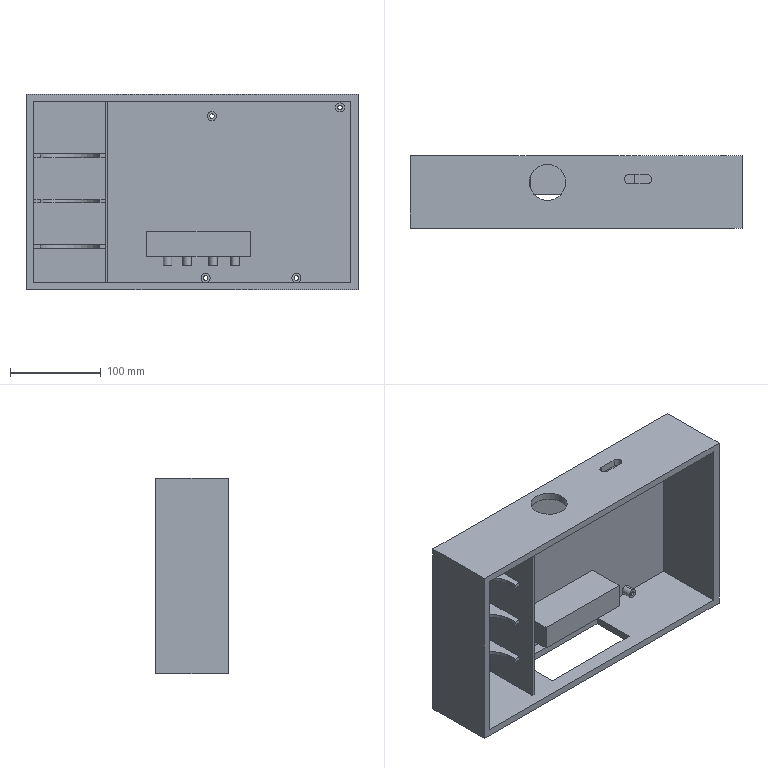Part | SolidWorks | features ICE 13, BossThin 1, Extrusion 1, LPattern 1 | 1 solid | 87 faces | box 366 x 80 x 216 mm | volume 981778 mm3 | plane 49 | cylinder 38 | commonest cylinder face diameters 10 x11 66.944 x9 5 x8 9.441 x8 40 x2